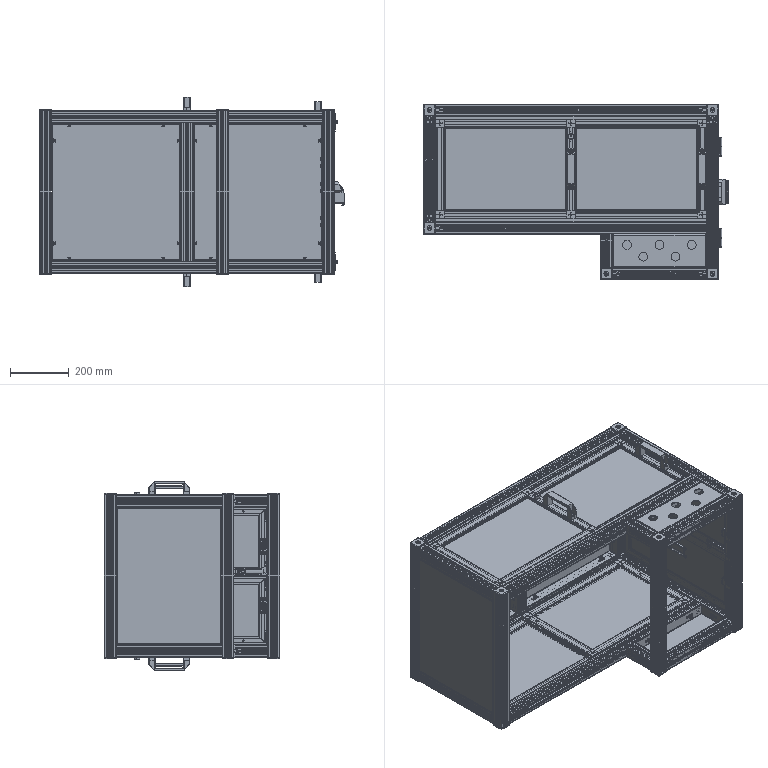Part | NX | features BREP 117 | 677 solids | 21924 faces | volume 14693918 mm3 | plane 13801 | cylinder 6219 | cone 1320 | torus 438 | sphere 90 | spline 56 | commonest cylinder face diameters 5 x744 8 x576 2 x453 0.562 x440 1 x399 6 x354